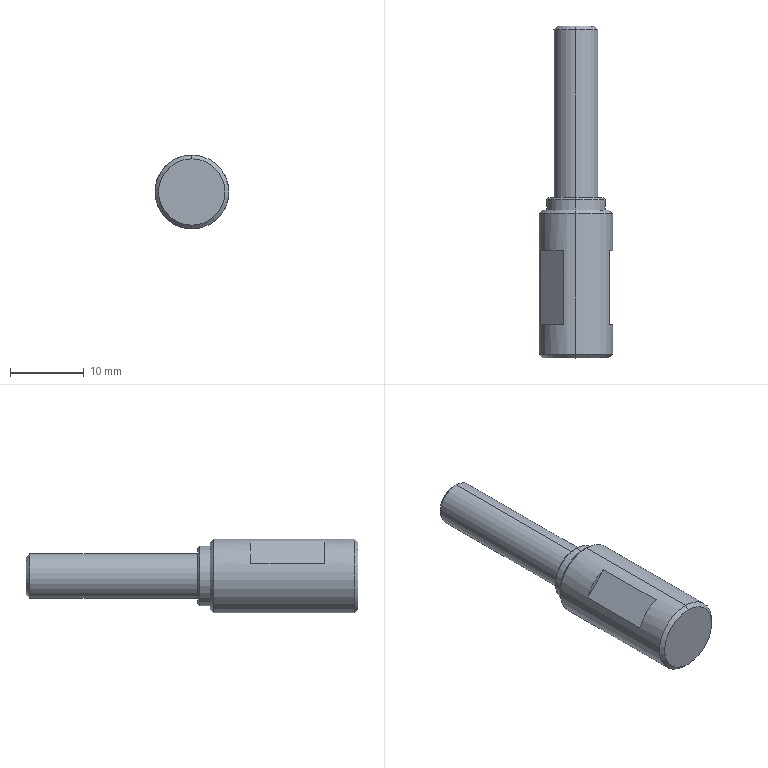Part | SolidWorks | features ICE 5, Chamfer 3, CirPattern 1, Extrusion 1 | 1 solid | 24 faces | box 10 x 44.9 x 10 mm | volume 2272 mm3 | plane 10 | cone 8 | cylinder 6 | commonest cylinder face diameters 6 x2 8 x2 10 x2
STEP:
#1=CARTESIAN_POINT('',(0.,20.,4.5));
#2=VERTEX_POINT('',#1);
#3=CARTESIAN_POINT('',(0.,20.,-4.5));
#4=VERTEX_POINT('',#3);
#5=CARTESIAN_POINT('',(0.,20.,0.));
#6=DIRECTION('',(0.,1.,0.));
#7=DIRECTION('',(0.,0.,-1.));
#8=AXIS2_PLACEMENT_3D('',#5,#6,#7);
#9=CIRCLE('',#8,4.5);
#10=EDGE_CURVE('',#2,#4,#9,.T.);
#11=ORIENTED_EDGE('',*,*,#10,.F.);
#12=CARTESIAN_POINT('',(0.,19.5,5.));
#13=VERTEX_POINT('',#12);
#14=CARTESIAN_POINT('',(0.,19.5,5.));
#15=DIRECTION('',(0.,-0.7071,0.7071));
#16=VECTOR('',#15,1000.);
#17=LINE('',#14,#16);
#18=EDGE_CURVE('',#2,#13,#17,.T.);
#19=ORIENTED_EDGE('',*,*,#18,.T.);
#20=CARTESIAN_POINT('',(0.,19.5,-5.));
#21=VERTEX_POINT('',#20);
#22=CARTESIAN_POINT('',(0.,19.5,0.));
#23=DIRECTION('',(0.,-1.,0.));
#24=DIRECTION('',(0.,0.,-1.));
#25=AXIS2_PLACEMENT_3D('',#22,#23,#24);
#26=CIRCLE('',#25,5.);
#27=EDGE_CURVE('',#21,#13,#26,.T.);
#28=ORIENTED_EDGE('',*,*,#27,.F.);
#29=CARTESIAN_POINT('',(0.,19.5,-5.));
#30=DIRECTION('',(0.,-0.7071,-0.7071));
#31=VECTOR('',#30,1000.);
#32=LINE('',#29,#31);
#33=EDGE_CURVE('',#4,#21,#32,.T.);
#34=ORIENTED_EDGE('',*,*,#33,.F.);
#35=EDGE_LOOP('',(#11,#19,#28,#34));
#36=FACE_OUTER_BOUND('',#35,.T.);
#37=CARTESIAN_POINT('',(0.,19.5,0.));
#38=DIRECTION('',(0.,-1.,0.));
#39=DIRECTION('',(0.,0.,-1.));
#40=AXIS2_PLACEMENT_3D('',#37,#38,#39);
#41=CONICAL_SURFACE('',#40,5.,0.7854);
#42=ADVANCED_FACE('',(#36),#41,.T.);
#43=CARTESIAN_POINT('',(0.,0.,-4.5));
#44=VERTEX_POINT('',#43);
#45=CARTESIAN_POINT('',(0.,0.,4.5));
#46=VERTEX_POINT('',#45);
#47=CARTESIAN_POINT('',(0.,0.,0.));
#48=DIRECTION('',(0.,-1.,0.));
#49=DIRECTION('',(0.,0.,1.));
#50=AXIS2_PLACEMENT_3D('',#47,#48,#49);
#51=CIRCLE('',#50,4.5);
#52=EDGE_CURVE('',#44,#46,#51,.T.);
#53=ORIENTED_EDGE('',*,*,#52,.F.);
#54=CARTESIAN_POINT('',(0.,0.5,-5.));
#55=VERTEX_POINT('',#54);
#56=CARTESIAN_POINT('',(0.,0.,-4.5));
#57=DIRECTION('',(0.,0.7071,-0.7071));
#58=VECTOR('',#57,1000.);
#59=LINE('',#56,#58);
#60=EDGE_CURVE('',#44,#55,#59,.T.);
#61=ORIENTED_EDGE('',*,*,#60,.T.);
#62=CARTESIAN_POINT('',(0.,0.5,5.));
#63=VERTEX_POINT('',#62);
#64=CARTESIAN_POINT('',(0.,0.5,0.));
#65=DIRECTION('',(0.,1.,0.));
#66=DIRECTION('',(0.,0.,1.));
#67=AXIS2_PLACEMENT_3D('',#64,#65,#66);
#68=CIRCLE('',#67,5.);
#69=EDGE_CURVE('',#63,#55,#68,.T.);
#70=ORIENTED_EDGE('',*,*,#69,.F.);
#71=CARTESIAN_POINT('',(0.,0.,4.5));
#72=DIRECTION('',(0.,0.7071,0.7071));
#73=VECTOR('',#72,1000.);
#74=LINE('',#71,#73);
#75=EDGE_CURVE('',#46,#63,#74,.T.);
#76=ORIENTED_EDGE('',*,*,#75,.F.);
#77=EDGE_LOOP('',(#53,#61,#70,#76));
#78=FACE_OUTER_BOUND('',#77,.T.);
#79=CARTESIAN_POINT('',(0.,0.,0.));
#80=DIRECTION('',(0.,1.,0.));
#81=DIRECTION('',(0.,0.,1.));
#82=AXIS2_PLACEMENT_3D('',#79,#80,#81);
#83=CONICAL_SURFACE('',#82,4.5,0.7854);
#84=ADVANCED_FACE('',(#78),#83,.T.);
#85=CARTESIAN_POINT('',(4.5,4.5,2.179));
#86=VERTEX_POINT('',#85);
#87=CARTESIAN_POINT('',(4.5,4.5,-2.179));
#88=VERTEX_POINT('',#87);
#89=CARTESIAN_POINT('',(0.,4.5,0.));
#90=DIRECTION('',(0.,1.,0.));
#91=DIRECTION('',(0.,0.,-1.));
#92=AXIS2_PLACEMENT_3D('',#89,#90,#91);
#93=CIRCLE('',#92,5.);
#94=EDGE_CURVE('',#86,#88,#93,.T.);
#95=ORIENTED_EDGE('',*,*,#94,.F.);
#96=CARTESIAN_POINT('',(4.5,14.5,2.179));
#97=VERTEX_POINT('',#96);
#98=CARTESIAN_POINT('',(4.5,20.,2.179));
#99=DIRECTION('',(0.,-1.,0.));
#100=VECTOR('',#99,1000.);
#101=LINE('',#98,#100);
#102=EDGE_CURVE('',#97,#86,#101,.T.);
#103=ORIENTED_EDGE('',*,*,#102,.F.);
#104=CARTESIAN_POINT('',(4.5,14.5,-2.179));
#105=VERTEX_POINT('',#104);
#106=CARTESIAN_POINT('',(0.,14.5,0.));
#107=DIRECTION('',(0.,-1.,0.));
#108=DIRECTION('',(0.,0.,1.));
#109=AXIS2_PLACEMENT_3D('',#106,#107,#108);
#110=CIRCLE('',#109,5.);
#111=EDGE_CURVE('',#105,#97,#110,.T.);
#112=ORIENTED_EDGE('',*,*,#111,.F.);
#113=CARTESIAN_POINT('',(4.5,20.,-2.179));
#114=DIRECTION('',(0.,1.,0.));
#115=VECTOR('',#114,1000.);
#116=LINE('',#113,#115);
#117=EDGE_CURVE('',#88,#105,#116,.T.);
#118=ORIENTED_EDGE('',*,*,#117,.F.);
#119=EDGE_LOOP('',(#95,#103,#112,#118));
#120=FACE_BOUND('',#119,.T.);
#121=ORIENTED_EDGE('',*,*,#27,.T.);
#122=CARTESIAN_POINT('',(0.,20.,5.));
#123=DIRECTION('',(0.,-1.,0.));
#124=VECTOR('',#123,1000.);
#125=LINE('',#122,#124);
#126=EDGE_CURVE('',#13,#63,#125,.T.);
#127=ORIENTED_EDGE('',*,*,#126,.T.);
#128=ORIENTED_EDGE('',*,*,#69,.T.);
#129=CARTESIAN_POINT('',(0.,20.,-5.));
#130=DIRECTION('',(0.,-1.,0.));
#131=VECTOR('',#130,1000.);
#132=LINE('',#129,#131);
#133=EDGE_CURVE('',#21,#55,#132,.T.);
#134=ORIENTED_EDGE('',*,*,#133,.F.);
#135=EDGE_LOOP('',(#121,#127,#128,#134));
#136=FACE_OUTER_BOUND('',#135,.T.);
#137=CARTESIAN_POINT('',(0.,20.,0.));
#138=DIRECTION('',(0.,-1.,0.));
#139=DIRECTION('',(0.,0.,-1.));
#140=AXIS2_PLACEMENT_3D('',#137,#138,#139);
#141=CYLINDRICAL_SURFACE('',#140,5.);
#142=ADVANCED_FACE('',(#120,#136),#141,.T.);
#143=CARTESIAN_POINT('',(0.,21.7,3.7));
#144=VERTEX_POINT('',#143);
#145=CARTESIAN_POINT('',(0.,21.7,-3.7));
#146=VERTEX_POINT('',#145);
#147=CARTESIAN_POINT('',(0.,21.7,0.));
#148=DIRECTION('',(0.,1.,0.));
#149=DIRECTION('',(0.,0.,1.));
#150=AXIS2_PLACEMENT_3D('',#147,#148,#149);
#151=CIRCLE('',#150,3.7);
#152=EDGE_CURVE('',#144,#146,#151,.T.);
#153=ORIENTED_EDGE('',*,*,#152,.F.);
#154=CARTESIAN_POINT('',(0.,21.4,4.));
#155=VERTEX_POINT('',#154);
#156=CARTESIAN_POINT('',(0.,21.7,3.7));
#157=DIRECTION('',(0.,-0.7071,0.7071));
#158=VECTOR('',#157,1000.);
#159=LINE('',#156,#158);
#160=EDGE_CURVE('',#144,#155,#159,.T.);
#161=ORIENTED_EDGE('',*,*,#160,.T.);
#162=CARTESIAN_POINT('',(0.,21.4,-4.));
#163=VERTEX_POINT('',#162);
#164=CARTESIAN_POINT('',(0.,21.4,0.));
#165=DIRECTION('',(0.,-1.,0.));
#166=DIRECTION('',(0.,0.,1.));
#167=AXIS2_PLACEMENT_3D('',#164,#165,#166);
#168=CIRCLE('',#167,4.);
#169=EDGE_CURVE('',#163,#155,#168,.T.);
#170=ORIENTED_EDGE('',*,*,#169,.F.);
#171=CARTESIAN_POINT('',(0.,21.7,-3.7));
#172=DIRECTION('',(0.,-0.7071,-0.7071));
#173=VECTOR('',#172,1000.);
#174=LINE('',#171,#173);
#175=EDGE_CURVE('',#146,#163,#174,.T.);
#176=ORIENTED_EDGE('',*,*,#175,.F.);
#177=EDGE_LOOP('',(#153,#161,#170,#176));
#178=FACE_OUTER_BOUND('',#177,.T.);
#179=CARTESIAN_POINT('',(0.,21.7,0.));
#180=DIRECTION('',(0.,-1.,0.));
#181=DIRECTION('',(0.,0.,-1.));
#182=AXIS2_PLACEMENT_3D('',#179,#180,#181);
#183=CONICAL_SURFACE('',#182,3.7,0.7854);
#184=ADVANCED_FACE('',(#178),#183,.T.);
#185=CARTESIAN_POINT('',(0.,44.9,2.5));
#186=VERTEX_POINT('',#185);
#187=CARTESIAN_POINT('',(0.,44.9,-2.5));
#188=VERTEX_POINT('',#187);
#189=CARTESIAN_POINT('',(0.,44.9,0.));
#190=DIRECTION('',(0.,1.,0.));
#191=DIRECTION('',(0.,0.,1.));
#192=AXIS2_PLACEMENT_3D('',#189,#190,#191);
#193=CIRCLE('',#192,2.5);
#194=EDGE_CURVE('',#186,#188,#193,.T.);
#195=ORIENTED_EDGE('',*,*,#194,.F.);
#196=CARTESIAN_POINT('',(0.,44.4,3.));
#197=VERTEX_POINT('',#196);
#198=CARTESIAN_POINT('',(0.,44.9,2.5));
#199=DIRECTION('',(0.,-0.7071,0.7071));
#200=VECTOR('',#199,1000.);
#201=LINE('',#198,#200);
#202=EDGE_CURVE('',#186,#197,#201,.T.);
#203=ORIENTED_EDGE('',*,*,#202,.T.);
#204=CARTESIAN_POINT('',(0.,44.4,-3.));
#205=VERTEX_POINT('',#204);
#206=CARTESIAN_POINT('',(0.,44.4,0.));
#207=DIRECTION('',(0.,-1.,0.));
#208=DIRECTION('',(0.,0.,1.));
#209=AXIS2_PLACEMENT_3D('',#206,#207,#208);
#210=CIRCLE('',#209,3.);
#211=EDGE_CURVE('',#205,#197,#210,.T.);
#212=ORIENTED_EDGE('',*,*,#211,.F.);
#213=CARTESIAN_POINT('',(0.,44.9,-2.5));
#214=DIRECTION('',(0.,-0.7071,-0.7071));
#215=VECTOR('',#214,1000.);
#216=LINE('',#213,#215);
#217=EDGE_CURVE('',#188,#205,#216,.T.);
#218=ORIENTED_EDGE('',*,*,#217,.F.);
#219=EDGE_LOOP('',(#195,#203,#212,#218));
#220=FACE_OUTER_BOUND('',#219,.T.);
#221=CARTESIAN_POINT('',(0.,44.9,0.));
#222=DIRECTION('',(0.,-1.,0.));
#223=DIRECTION('',(0.,0.,-1.));
#224=AXIS2_PLACEMENT_3D('',#221,#222,#223);
#225=CONICAL_SURFACE('',#224,2.5,0.7854);
#226=ADVANCED_FACE('',(#220),#225,.T.);
#227=ORIENTED_EDGE('',*,*,#211,.T.);
#228=CARTESIAN_POINT('',(0.,21.7,3.));
#229=VERTEX_POINT('',#228);
#230=CARTESIAN_POINT('',(0.,44.9,3.));
#231=DIRECTION('',(0.,-1.,0.));
#232=VECTOR('',#231,1000.);
#233=LINE('',#230,#232);
#234=EDGE_CURVE('',#197,#229,#233,.T.);
#235=ORIENTED_EDGE('',*,*,#234,.T.);
#236=CARTESIAN_POINT('',(0.,21.7,-3.));
#237=VERTEX_POINT('',#236);
#238=CARTESIAN_POINT('',(0.,21.7,0.));
#239=DIRECTION('',(0.,1.,0.));
#240=DIRECTION('',(0.,0.,1.));
#241=AXIS2_PLACEMENT_3D('',#238,#239,#240);
#242=CIRCLE('',#241,3.);
#243=EDGE_CURVE('',#229,#237,#242,.T.);
#244=ORIENTED_EDGE('',*,*,#243,.T.);
#245=CARTESIAN_POINT('',(0.,44.9,-3.));
#246=DIRECTION('',(0.,-1.,0.));
#247=VECTOR('',#246,1000.);
#248=LINE('',#245,#247);
#249=EDGE_CURVE('',#205,#237,#248,.T.);
#250=ORIENTED_EDGE('',*,*,#249,.F.);
#251=EDGE_LOOP('',(#227,#235,#244,#250));
#252=FACE_OUTER_BOUND('',#251,.T.);
#253=CARTESIAN_POINT('',(0.,44.9,0.));
#254=DIRECTION('',(0.,-1.,0.));
#255=DIRECTION('',(0.,0.,-1.));
#256=AXIS2_PLACEMENT_3D('',#253,#254,#255);
#257=CYLINDRICAL_SURFACE('',#256,3.);
#258=ADVANCED_FACE('',(#252),#257,.T.);
#259=ORIENTED_EDGE('',*,*,#169,.T.);
#260=CARTESIAN_POINT('',(0.,20.,4.));
#261=VERTEX_POINT('',#260);
#262=CARTESIAN_POINT('',(0.,21.7,4.));
#263=DIRECTION('',(0.,-1.,0.));
#264=VECTOR('',#263,1000.);
#265=LINE('',#262,#264);
#266=EDGE_CURVE('',#155,#261,#265,.T.);
#267=ORIENTED_EDGE('',*,*,#266,.T.);
#268=CARTESIAN_POINT('',(0.,20.,-4.));
#269=VERTEX_POINT('',#268);
#270=CARTESIAN_POINT('',(0.,20.,0.));
#271=DIRECTION('',(0.,-1.,0.));
#272=DIRECTION('',(0.,0.,-1.));
#273=AXIS2_PLACEMENT_3D('',#270,#271,#272);
#274=CIRCLE('',#273,4.);
#275=EDGE_CURVE('',#269,#261,#274,.T.);
#276=ORIENTED_EDGE('',*,*,#275,.F.);
#277=CARTESIAN_POINT('',(0.,21.7,-4.));
#278=DIRECTION('',(0.,-1.,0.));
#279=VECTOR('',#278,1000.);
#280=LINE('',#277,#279);
#281=EDGE_CURVE('',#163,#269,#280,.T.);
#282=ORIENTED_EDGE('',*,*,#281,.F.);
#283=EDGE_LOOP('',(#259,#267,#276,#282));
#284=FACE_OUTER_BOUND('',#283,.T.);
#285=CARTESIAN_POINT('',(0.,21.7,0.));
#286=DIRECTION('',(0.,-1.,0.));
#287=DIRECTION('',(0.,0.,-1.));
#288=AXIS2_PLACEMENT_3D('',#285,#286,#287);
#289=CYLINDRICAL_SURFACE('',#288,4.);
#290=ADVANCED_FACE('',(#284),#289,.T.);
#291=ORIENTED_EDGE('',*,*,#266,.F.);
#292=CARTESIAN_POINT('',(0.,21.4,0.));
#293=DIRECTION('',(0.,-1.,0.));
#294=DIRECTION('',(0.,0.,1.));
#295=AXIS2_PLACEMENT_3D('',#292,#293,#294);
#296=CIRCLE('',#295,4.);
#297=EDGE_CURVE('',#155,#163,#296,.T.);
#298=ORIENTED_EDGE('',*,*,#297,.T.);
#299=ORIENTED_EDGE('',*,*,#281,.T.);
#300=CARTESIAN_POINT('',(0.,20.,0.));
#301=DIRECTION('',(0.,-1.,0.));
#302=DIRECTION('',(0.,0.,-1.));
#303=AXIS2_PLACEMENT_3D('',#300,#301,#302);
#304=CIRCLE('',#303,4.);
#305=EDGE_CURVE('',#261,#269,#304,.T.);
#306=ORIENTED_EDGE('',*,*,#305,.F.);
#307=EDGE_LOOP('',(#291,#298,#299,#306));
#308=FACE_OUTER_BOUND('',#307,.T.);
#309=CARTESIAN_POINT('',(0.,21.7,0.));
#310=DIRECTION('',(0.,-1.,0.));
#311=DIRECTION('',(0.,0.,-1.));
#312=AXIS2_PLACEMENT_3D('',#309,#310,#311);
#313=CYLINDRICAL_SURFACE('',#312,4.);
#314=ADVANCED_FACE('',(#308),#313,.T.);
#315=CARTESIAN_POINT('',(0.,21.7,0.));
#316=DIRECTION('',(0.,1.,0.));
#317=DIRECTION('',(0.,0.,1.));
#318=AXIS2_PLACEMENT_3D('',#315,#316,#317);
#319=CIRCLE('',#318,3.7);
#320=EDGE_CURVE('',#146,#144,#319,.T.);
#321=ORIENTED_EDGE('',*,*,#320,.T.);
#322=ORIENTED_EDGE('',*,*,#152,.T.);
#323=EDGE_LOOP('',(#321,#322));
#324=FACE_OUTER_BOUND('',#323,.T.);
#325=CARTESIAN_POINT('',(0.,21.7,0.));
#326=DIRECTION('',(0.,1.,0.));
#327=DIRECTION('',(0.,0.,1.));
#328=AXIS2_PLACEMENT_3D('',#325,#326,#327);
#329=CIRCLE('',#328,3.);
#330=EDGE_CURVE('',#237,#229,#329,.T.);
#331=ORIENTED_EDGE('',*,*,#330,.F.);
#332=ORIENTED_EDGE('',*,*,#243,.F.);
#333=EDGE_LOOP('',(#331,#332));
#334=FACE_BOUND('',#333,.T.);
#335=CARTESIAN_POINT('',(0.,21.7,0.));
#336=DIRECTION('',(0.,1.,0.));
#337=DIRECTION('',(0.,0.,1.));
#338=AXIS2_PLACEMENT_3D('',#335,#336,#337);
#339=PLANE('',#338);
#340=ADVANCED_FACE('',(#324,#334),#339,.T.);
#341=ORIENTED_EDGE('',*,*,#234,.F.);
#342=CARTESIAN_POINT('',(0.,44.4,0.));
#343=DIRECTION('',(0.,-1.,0.));
#344=DIRECTION('',(0.,0.,1.));
#345=AXIS2_PLACEMENT_3D('',#342,#343,#344);
#346=CIRCLE('',#345,3.);
#347=EDGE_CURVE('',#197,#205,#346,.T.);
#348=ORIENTED_EDGE('',*,*,#347,.T.);
#349=ORIENTED_EDGE('',*,*,#249,.T.);
#350=ORIENTED_EDGE('',*,*,#330,.T.);
#351=EDGE_LOOP('',(#341,#348,#349,#350));
#352=FACE_OUTER_BOUND('',#351,.T.);
#353=CARTESIAN_POINT('',(0.,44.9,0.));
#354=DIRECTION('',(0.,-1.,0.));
#355=DIRECTION('',(0.,0.,-1.));
#356=AXIS2_PLACEMENT_3D('',#353,#354,#355);
#357=CYLINDRICAL_SURFACE('',#356,3.);
#358=ADVANCED_FACE('',(#352),#357,.T.);
#359=CARTESIAN_POINT('',(0.,44.9,0.));
#360=DIRECTION('',(0.,1.,0.));
#361=DIRECTION('',(0.,0.,1.));
#362=AXIS2_PLACEMENT_3D('',#359,#360,#361);
#363=CIRCLE('',#362,2.5);
#364=EDGE_CURVE('',#188,#186,#363,.T.);
#365=ORIENTED_EDGE('',*,*,#364,.T.);
#366=ORIENTED_EDGE('',*,*,#194,.T.);
#367=EDGE_LOOP('',(#365,#366));
#368=FACE_OUTER_BOUND('',#367,.T.);
#369=CARTESIAN_POINT('',(0.,44.9,0.));
#370=DIRECTION('',(0.,1.,0.));
#371=DIRECTION('',(0.,0.,1.));
#372=AXIS2_PLACEMENT_3D('',#369,#370,#371);
#373=PLANE('',#372);
#374=ADVANCED_FACE('',(#368),#373,.T.);
#375=ORIENTED_EDGE('',*,*,#202,.F.);
#376=ORIENTED_EDGE('',*,*,#364,.F.);
#377=ORIENTED_EDGE('',*,*,#217,.T.);
#378=ORIENTED_EDGE('',*,*,#347,.F.);
#379=EDGE_LOOP('',(#375,#376,#377,#378));
#380=FACE_OUTER_BOUND('',#379,.T.);
#381=CARTESIAN_POINT('',(0.,44.9,0.));
#382=DIRECTION('',(0.,-1.,0.));
#383=DIRECTION('',(0.,0.,-1.));
#384=AXIS2_PLACEMENT_3D('',#381,#382,#383);
#385=CONICAL_SURFACE('',#384,2.5,0.7854);
#386=ADVANCED_FACE('',(#380),#385,.T.);
#387=ORIENTED_EDGE('',*,*,#160,.F.);
#388=ORIENTED_EDGE('',*,*,#320,.F.);
#389=ORIENTED_EDGE('',*,*,#175,.T.);
#390=ORIENTED_EDGE('',*,*,#297,.F.);
#391=EDGE_LOOP('',(#387,#388,#389,#390));
#392=FACE_OUTER_BOUND('',#391,.T.);
#393=CARTESIAN_POINT('',(0.,21.7,0.));
#394=DIRECTION('',(0.,-1.,0.));
#395=DIRECTION('',(0.,0.,-1.));
#396=AXIS2_PLACEMENT_3D('',#393,#394,#395);
#397=CONICAL_SURFACE('',#396,3.7,0.7854);
#398=ADVANCED_FACE('',(#392),#397,.T.);
#399=CARTESIAN_POINT('',(0.,20.,0.));
#400=DIRECTION('',(0.,1.,0.));
#401=DIRECTION('',(0.,0.,-1.));
#402=AXIS2_PLACEMENT_3D('',#399,#400,#401);
#403=CIRCLE('',#402,4.5);
#404=EDGE_CURVE('',#4,#2,#403,.T.);
#405=ORIENTED_EDGE('',*,*,#404,.T.);
#406=ORIENTED_EDGE('',*,*,#10,.T.);
#407=EDGE_LOOP('',(#405,#406));
#408=FACE_OUTER_BOUND('',#407,.T.);
#409=ORIENTED_EDGE('',*,*,#275,.T.);
#410=ORIENTED_EDGE('',*,*,#305,.T.);
#411=EDGE_LOOP('',(#409,#410));
#412=FACE_BOUND('',#411,.T.);
#413=CARTESIAN_POINT('',(0.,20.,0.));
#414=DIRECTION('',(0.,-1.,0.));
#415=DIRECTION('',(0.,0.,-1.));
#416=AXIS2_PLACEMENT_3D('',#413,#414,#415);
#417=PLANE('',#416);
#418=ADVANCED_FACE('',(#408,#412),#417,.F.);
#419=ORIENTED_EDGE('',*,*,#126,.F.);
#420=CARTESIAN_POINT('',(0.,19.5,0.));
#421=DIRECTION('',(0.,-1.,0.));
#422=DIRECTION('',(0.,0.,-1.));
#423=AXIS2_PLACEMENT_3D('',#420,#421,#422);
#424=CIRCLE('',#423,5.);
#425=EDGE_CURVE('',#13,#21,#424,.T.);
#426=ORIENTED_EDGE('',*,*,#425,.T.);
#427=ORIENTED_EDGE('',*,*,#133,.T.);
#428=CARTESIAN_POINT('',(0.,0.5,0.));
#429=DIRECTION('',(0.,1.,0.));
#430=DIRECTION('',(0.,0.,1.));
#431=AXIS2_PLACEMENT_3D('',#428,#429,#430);
#432=CIRCLE('',#431,5.);
#433=EDGE_CURVE('',#55,#63,#432,.T.);
#434=ORIENTED_EDGE('',*,*,#433,.T.);
#435=EDGE_LOOP('',(#419,#426,#427,#434));
#436=FACE_OUTER_BOUND('',#435,.T.);
#437=CARTESIAN_POINT('',(-4.723,4.5,1.641));
#438=VERTEX_POINT('',#437);
#439=CARTESIAN_POINT('',(-1.641,4.5,4.723));
#440=VERTEX_POINT('',#439);
#441=CARTESIAN_POINT('',(0.,4.5,0.));
#442=DIRECTION('',(0.,1.,0.));
#443=DIRECTION('',(0.,0.,-1.));
#444=AXIS2_PLACEMENT_3D('',#441,#442,#443);
#445=CIRCLE('',#444,5.);
#446=EDGE_CURVE('',#438,#440,#445,.T.);
#447=ORIENTED_EDGE('',*,*,#446,.F.);
#448=CARTESIAN_POINT('',(-4.723,14.5,1.641));
#449=VERTEX_POINT('',#448);
#450=CARTESIAN_POINT('',(-4.723,20.,1.641));
#451=DIRECTION('',(0.,-1.,0.));
#452=VECTOR('',#451,1000.);
#453=LINE('',#450,#452);
#454=EDGE_CURVE('',#449,#438,#453,.T.);
#455=ORIENTED_EDGE('',*,*,#454,.F.);
#456=CARTESIAN_POINT('',(-1.641,14.5,4.723));
#457=VERTEX_POINT('',#456);
#458=CARTESIAN_POINT('',(0.,14.5,0.));
#459=DIRECTION('',(0.,-1.,0.));
#460=DIRECTION('',(0.,0.,1.));
#461=AXIS2_PLACEMENT_3D('',#458,#459,#460);
#462=CIRCLE('',#461,5.);
#463=EDGE_CURVE('',#457,#449,#462,.T.);
#464=ORIENTED_EDGE('',*,*,#463,.F.);
#465=CARTESIAN_POINT('',(-1.641,20.,4.723));
#466=DIRECTION('',(0.,1.,0.));
#467=VECTOR('',#466,1000.);
#468=LINE('',#465,#467);
#469=EDGE_CURVE('',#440,#457,#468,.T.);
#470=ORIENTED_EDGE('',*,*,#469,.F.);
#471=EDGE_LOOP('',(#447,#455,#464,#470));
#472=FACE_BOUND('',#471,.T.);
#473=CARTESIAN_POINT('',(0.,20.,0.));
#474=DIRECTION('',(0.,-1.,0.));
#475=DIRECTION('',(0.,0.,-1.));
#476=AXIS2_PLACEMENT_3D('',#473,#474,#475);
#477=CYLINDRICAL_SURFACE('',#476,5.);
#478=ADVANCED_FACE('',(#436,#472),#477,.T.);
#479=CARTESIAN_POINT('',(0.,0.,0.));
#480=DIRECTION('',(0.,-1.,0.));
#481=DIRECTION('',(0.,0.,1.));
#482=AXIS2_PLACEMENT_3D('',#479,#480,#481);
#483=CIRCLE('',#482,4.5);
#484=EDGE_CURVE('',#46,#44,#483,.T.);
#485=ORIENTED_EDGE('',*,*,#484,.T.);
#486=ORIENTED_EDGE('',*,*,#52,.T.);
#487=EDGE_LOOP('',(#485,#486));
#488=FACE_OUTER_BOUND('',#487,.T.);
#489=CARTESIAN_POINT('',(0.,0.,0.));
#490=DIRECTION('',(0.,1.,0.));
#491=DIRECTION('',(0.,0.,1.));
#492=AXIS2_PLACEMENT_3D('',#489,#490,#491);
#493=PLANE('',#492);
#494=ADVANCED_FACE('',(#488),#493,.F.);
#495=ORIENTED_EDGE('',*,*,#60,.F.);
#496=ORIENTED_EDGE('',*,*,#484,.F.);
#497=ORIENTED_EDGE('',*,*,#75,.T.);
#498=ORIENTED_EDGE('',*,*,#433,.F.);
#499=EDGE_LOOP('',(#495,#496,#497,#498));
#500=FACE_OUTER_BOUND('',#499,.T.);
#501=CARTESIAN_POINT('',(0.,0.,0.));
#502=DIRECTION('',(0.,1.,0.));
#503=DIRECTION('',(0.,0.,1.));
#504=AXIS2_PLACEMENT_3D('',#501,#502,#503);
#505=CONICAL_SURFACE('',#504,4.5,0.7854);
#506=ADVANCED_FACE('',(#500),#505,.T.);
#507=ORIENTED_EDGE('',*,*,#18,.F.);
#508=ORIENTED_EDGE('',*,*,#404,.F.);
#509=ORIENTED_EDGE('',*,*,#33,.T.);
#510=ORIENTED_EDGE('',*,*,#425,.F.);
#511=EDGE_LOOP('',(#507,#508,#509,#510));
#512=FACE_OUTER_BOUND('',#511,.T.);
#513=CARTESIAN_POINT('',(0.,19.5,0.));
#514=DIRECTION('',(0.,-1.,0.));
#515=DIRECTION('',(0.,0.,-1.));
#516=AXIS2_PLACEMENT_3D('',#513,#514,#515);
#517=CONICAL_SURFACE('',#516,5.,0.7854);
#518=ADVANCED_FACE('',(#512),#517,.T.);
#519=ORIENTED_EDGE('',*,*,#94,.T.);
#520=CARTESIAN_POINT('',(4.5,4.5,-10.));
#521=DIRECTION('',(0.,0.,1.));
#522=VECTOR('',#521,1000.);
#523=LINE('',#520,#522);
#524=EDGE_CURVE('',#88,#86,#523,.T.);
#525=ORIENTED_EDGE('',*,*,#524,.T.);
#526=EDGE_LOOP('',(#519,#525));
#527=FACE_OUTER_BOUND('',#526,.T.);
#528=CARTESIAN_POINT('',(4.5,4.5,-10.));
#529=DIRECTION('',(0.,-1.,0.));
#530=DIRECTION('',(0.,0.,-1.));
#531=AXIS2_PLACEMENT_3D('',#528,#529,#530);
#532=PLANE('',#531);
#533=ADVANCED_FACE('',(#527),#532,.F.);
#534=ORIENTED_EDGE('',*,*,#117,.T.);
#535=CARTESIAN_POINT('',(4.5,14.5,-10.));
#536=DIRECTION('',(0.,0.,1.));
#537=VECTOR('',#536,1000.);
#538=LINE('',#535,#537);
#539=EDGE_CURVE('',#105,#97,#538,.T.);
#540=ORIENTED_EDGE('',*,*,#539,.T.);
#541=ORIENTED_EDGE('',*,*,#102,.T.);
#542=ORIENTED_EDGE('',*,*,#524,.F.);
#543=EDGE_LOOP('',(#534,#540,#541,#542));
#544=FACE_OUTER_BOUND('',#543,.T.);
#545=CARTESIAN_POINT('',(4.5,14.5,-10.));
#546=DIRECTION('',(-1.,0.,0.));
#547=DIRECTION('',(0.,-1.,0.));
#548=AXIS2_PLACEMENT_3D('',#545,#546,#547);
#549=PLANE('',#548);
#550=ADVANCED_FACE('',(#544),#549,.F.);
#551=ORIENTED_EDGE('',*,*,#111,.T.);
#552=ORIENTED_EDGE('',*,*,#539,.F.);
#553=EDGE_LOOP('',(#551,#552));
#554=FACE_OUTER_BOUND('',#553,.T.);
#555=CARTESIAN_POINT('',(4.5,14.5,-10.));
#556=DIRECTION('',(0.,1.,0.));
#557=DIRECTION('',(0.,0.,1.));
#558=AXIS2_PLACEMENT_3D('',#555,#556,#557);
#559=PLANE('',#558);
#560=ADVANCED_FACE('',(#554),#559,.F.);
#561=ORIENTED_EDGE('',*,*,#446,.T.);
#562=CARTESIAN_POINT('',(3.889,4.5,10.253));
#563=DIRECTION('',(-0.7071,0.,-0.7071));
#564=VECTOR('',#563,1000.);
#565=LINE('',#562,#564);
#566=EDGE_CURVE('',#440,#438,#565,.T.);
#567=ORIENTED_EDGE('',*,*,#566,.T.);
#568=EDGE_LOOP('',(#561,#567));
#569=FACE_OUTER_BOUND('',#568,.T.);
#570=CARTESIAN_POINT('',(3.889,4.5,10.253));
#571=DIRECTION('',(0.,-1.,0.));
#572=DIRECTION('',(0.,0.,-1.));
#573=AXIS2_PLACEMENT_3D('',#570,#571,#572);
#574=PLANE('',#573);
#575=ADVANCED_FACE('',(#569),#574,.F.);
#576=ORIENTED_EDGE('',*,*,#469,.T.);
#577=CARTESIAN_POINT('',(3.889,14.5,10.253));
#578=DIRECTION('',(-0.7071,0.,-0.7071));
#579=VECTOR('',#578,1000.);
#580=LINE('',#577,#579);
#581=EDGE_CURVE('',#457,#449,#580,.T.);
#582=ORIENTED_EDGE('',*,*,#581,.T.);
#583=ORIENTED_EDGE('',*,*,#454,.T.);
#584=ORIENTED_EDGE('',*,*,#566,.F.);
#585=EDGE_LOOP('',(#576,#582,#583,#584));
#586=FACE_OUTER_BOUND('',#585,.T.);
#587=CARTESIAN_POINT('',(3.889,14.5,10.253));
#588=DIRECTION('',(0.7071,0.,-0.7071));
#589=DIRECTION('',(-0.7071,0.,-0.7071));
#590=AXIS2_PLACEMENT_3D('',#587,#588,#589);
#591=PLANE('',#590);
#592=ADVANCED_FACE('',(#586),#591,.F.);
#593=ORIENTED_EDGE('',*,*,#463,.T.);
#594=ORIENTED_EDGE('',*,*,#581,.F.);
#595=EDGE_LOOP('',(#593,#594));
#596=FACE_OUTER_BOUND('',#595,.T.);
#597=CARTESIAN_POINT('',(3.889,14.5,10.253));
#598=DIRECTION('',(0.,1.,0.));
#599=DIRECTION('',(0.,0.,1.));
#600=AXIS2_PLACEMENT_3D('',#597,#598,#599);
#601=PLANE('',#600);
#602=ADVANCED_FACE('',(#596),#601,.F.);
#603=CLOSED_SHELL('',(#42,#84,#142,#184,#226,#258,#290,#314,#340,#358,#374,#386,#398,#418,#478,#494,#506,#518,#533,#550,#560,#575,#592,#602));
#604=MANIFOLD_SOLID_BREP('',#603);
#605=CARTESIAN_POINT('',(0.,0.,0.));
#606=DIRECTION('',(0.,0.,1.));
#607=DIRECTION('',(1.,0.,0.));
#608=AXIS2_PLACEMENT_3D('',#605,#606,#607);
#609=(LENGTH_UNIT()NAMED_UNIT(*)SI_UNIT(.MILLI.,.METRE.));
#610=UNCERTAINTY_MEASURE_WITH_UNIT(LENGTH_MEASURE(0.00001),#609,'','');
#611=(NAMED_UNIT(*)PLANE_ANGLE_UNIT()SI_UNIT($,.RADIAN.));
#612=(NAMED_UNIT(*)SI_UNIT($,.STERADIAN.)SOLID_ANGLE_UNIT());
#613=(GEOMETRIC_REPRESENTATION_CONTEXT(3)GLOBAL_UNCERTAINTY_ASSIGNED_CONTEXT((#610))GLOBAL_UNIT_ASSIGNED_CONTEXT((#609,#611,#612))REPRESENTATION_CONTEXT('',''));
#614=ADVANCED_BREP_SHAPE_REPRESENTATION('',(#604,#608),#613);